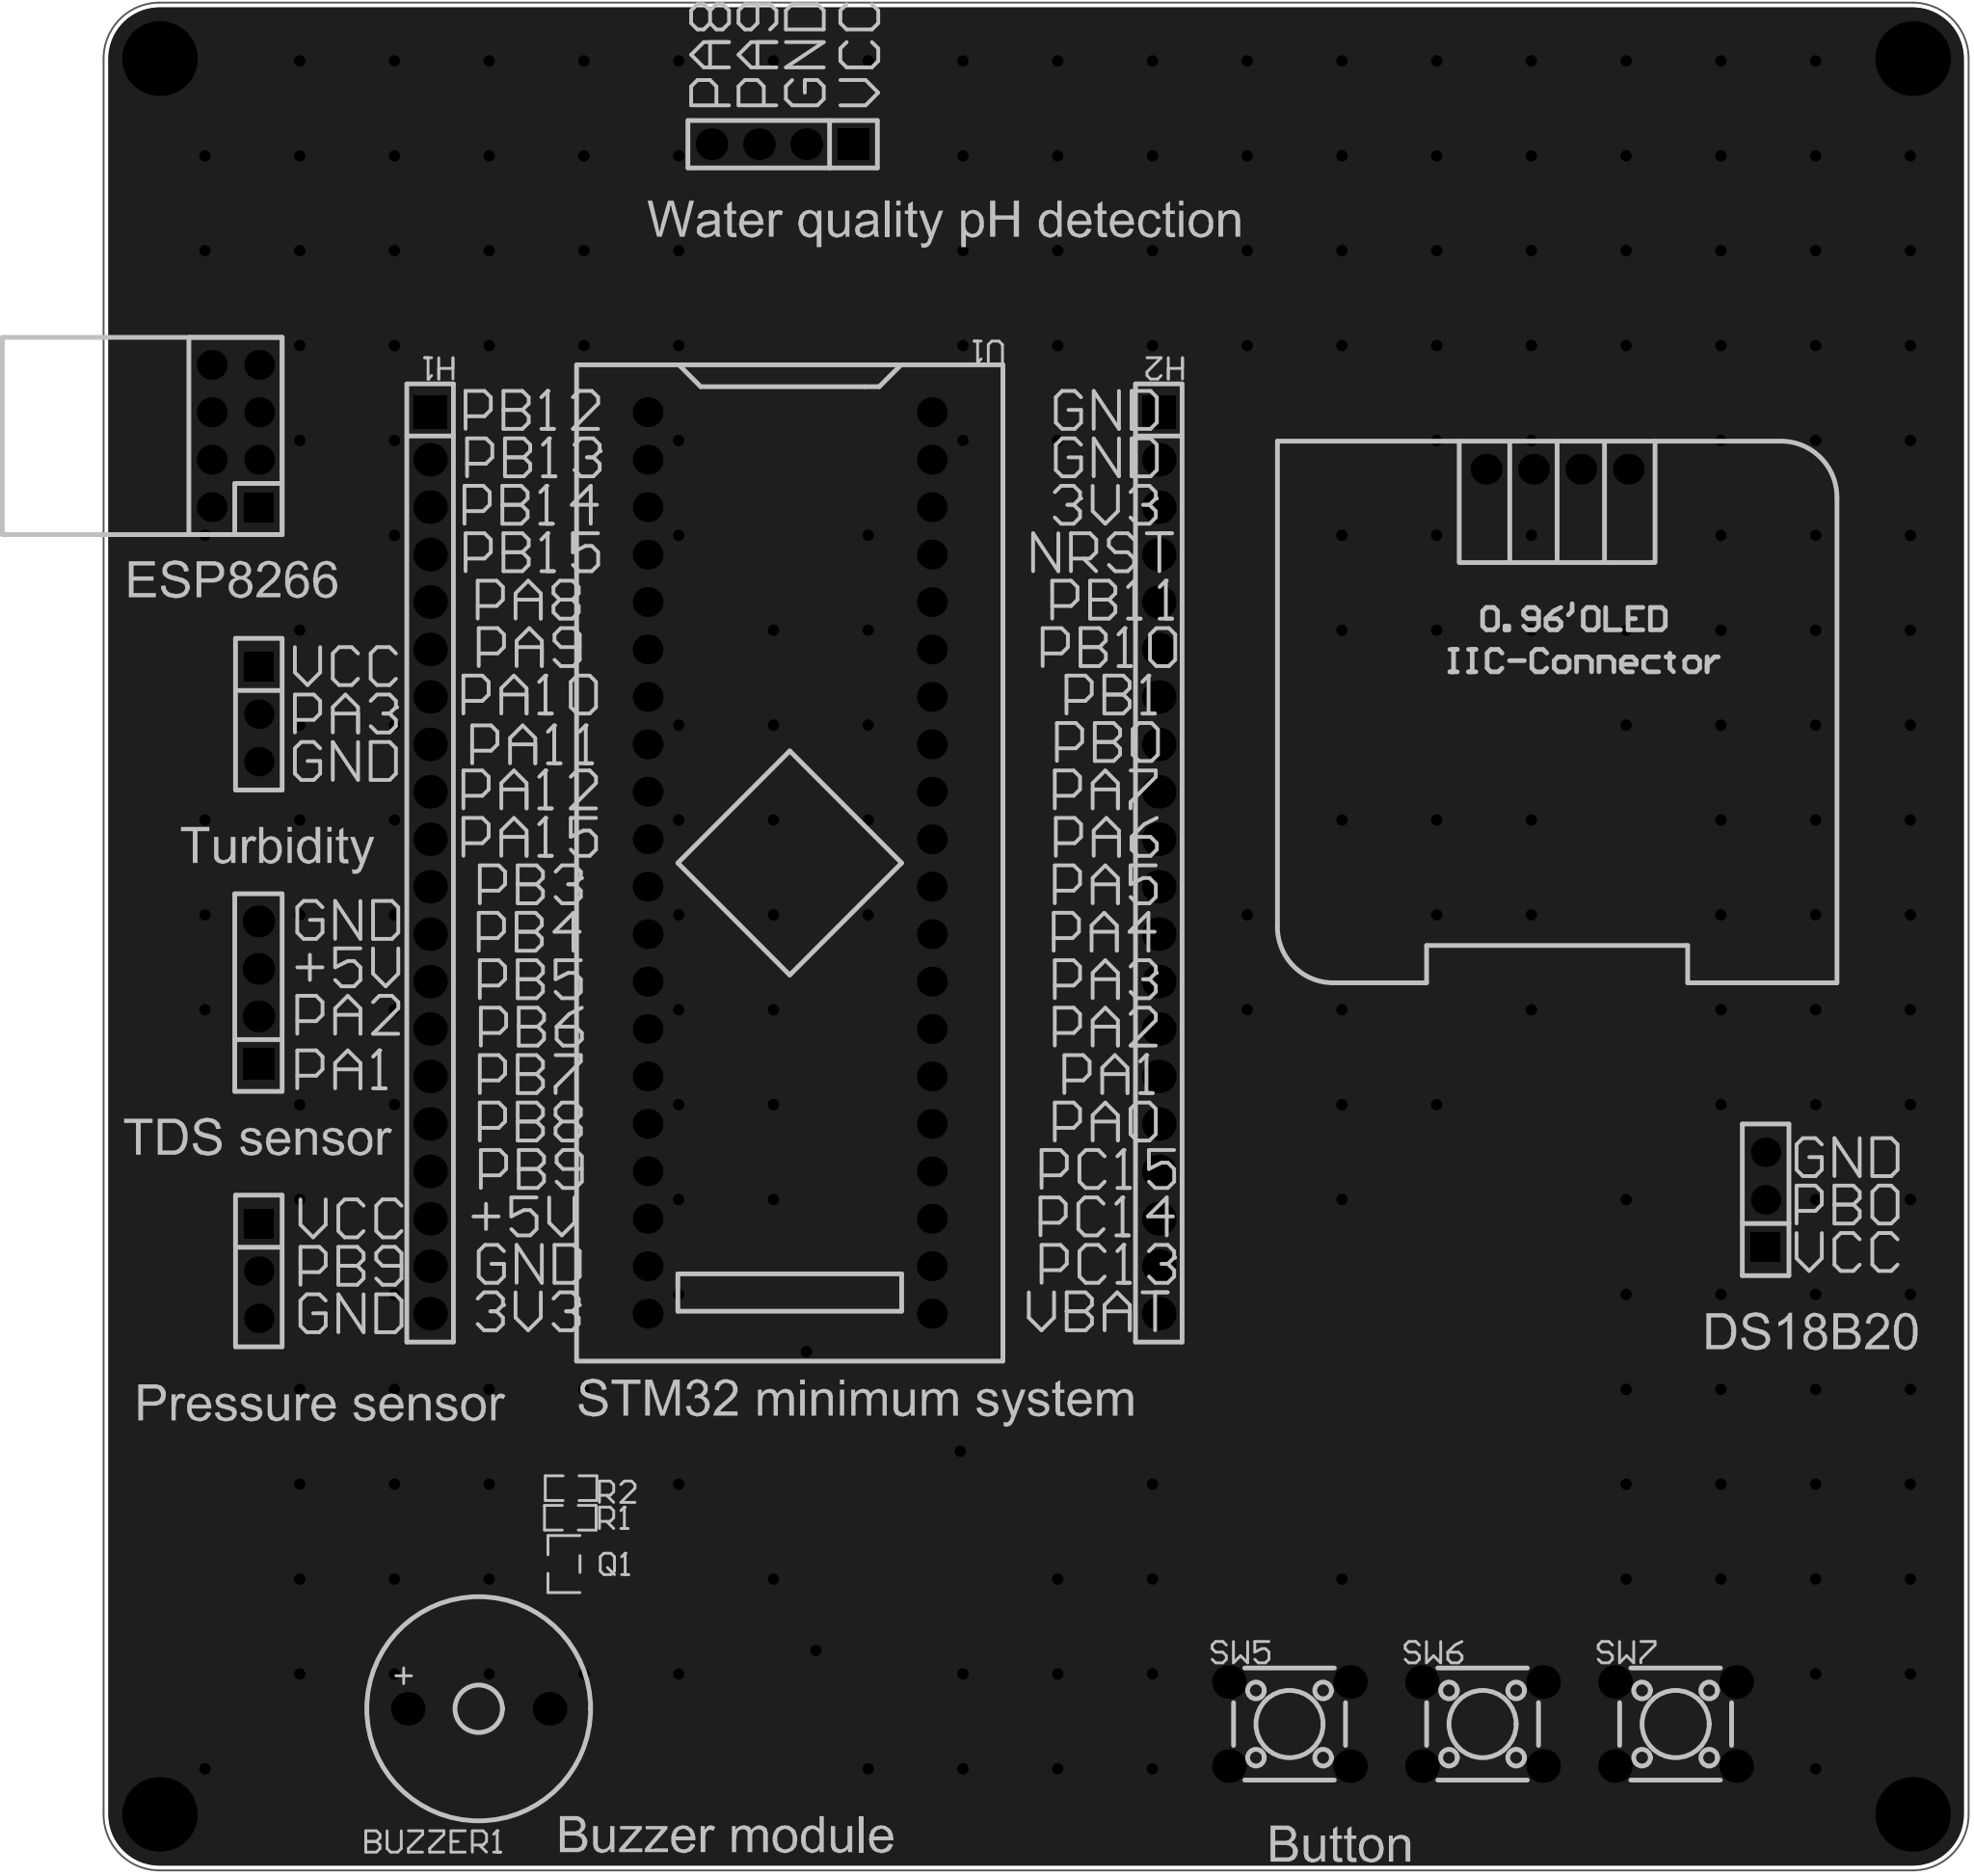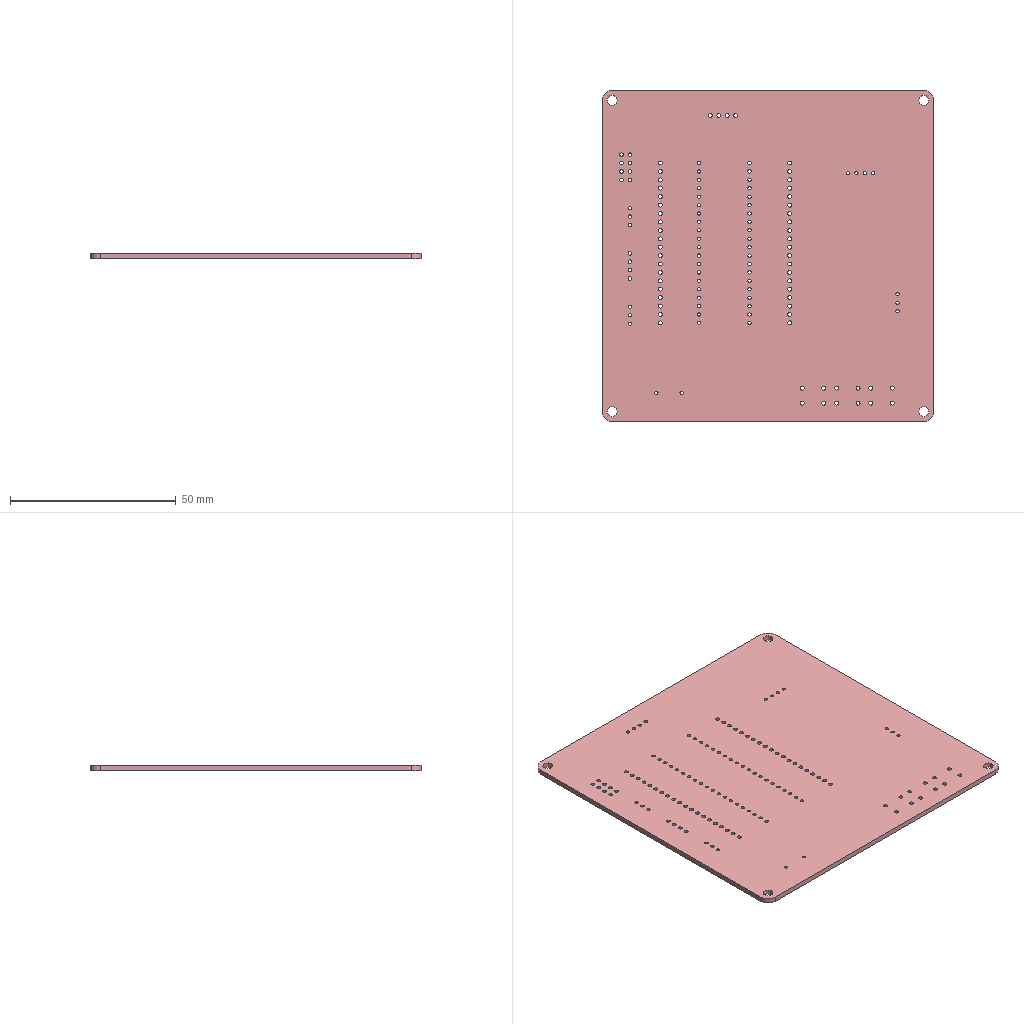Circuit board layout | Altium Designer | box 100 x 100 x 1.6 mm
Layer stack:
# Altium Designer layer stack of  (unit mm; dielectric type: 0 none, 1 core, 2 prepreg, 3 surface material)
index,name,kind,layer,copper_thickness_mm,dielectric_type,dielectric_thickness_mm,dielectric_material,dielectric_constant
0,Top Paste Mask Layer,other,,,,,,
1,Top Silkscreen Layer,other,,,,,,
2,Top Solder Mask Layer,dielectric,,,3,0.01,,3.3
3,Top Layer,copper,Top Layer,0.035,,,,
4,Dielectric1,dielectric,,,3,1.51,FR4,4.5
5,Bottom Layer,copper,Bottom Layer,0.035,,,,
6,Bottom Solder Mask Layer,dielectric,,,3,0.01,,3.3
7,Bottom Silkscreen Layer,other,,,,,,
8,Bottom Paste Mask Layer,other,,,,,,
# drill layer pairs: low layer,high layer
drill_pair,Top Layer,Bottom Layer
Part placement:
Designator,Comment,Layer,Footprint,Center-X(mm),Center-Y(mm),Rotation
U1,STM32F103C8T6-Card,TopLayer,CONN-TH_L53.3-W22.9_STM32F103C8T6-CARD,118.418,132.842,270
BUZZER1,buzzer-12X9,TopLayer,BUZ-TH_BD12.0-P7.60-D0.6-FD,101.74,87.559,0
H14,,TopLayer,HDR-TH_4P-P2.54-V-F,89.93,125.903,90
OLED1,,TopLayer,0.96OLED_4P,159.566,153.924,0
Q1,S8050 J3Y(RANGE:200-350),TopLayer,SOT-23-3_L3.0-W1.7-P0.95-LS2.9-BR,106.312,95.306,0
R1,10K,TopLayer,R0603,106.651,97.786,0
H15,,TopLayer,HDR-TH_3P-P2.54-V-F,170.742,114.808,90
H16,,TopLayer,HDR-TH_8P-P2.54-V-F-R2-C4-S2.54-1,88.7,155.702,90
H1,,TopLayer,HDR-TH_20P-P2.54-V-F,99.135,132.842,270
H2,,TopLayer,HDR-TH_20P-P2.54-V-F,138.206,132.842,270
H17,,TopLayer,HDR-TH_3P-P2.54-V-F,89.95,110.998,270
H18,,TopLayer,HDR-TH_3P-P2.54-V-F,89.95,140.807,270
R2,10K,TopLayer,R0603,106.693,99.37,180
SW5,,TopLayer,SW-TH_4P-L6.0-W6.0-P4.50-LS6.5,145.215,86.741,0
SW6,,TopLayer,SW-TH_4P-L6.0-W6.0-P4.50-LS6.5,155.565,86.741,0
SW7,,TopLayer,SW-TH_4P-L6.0-W6.0-P4.50-LS6.5,165.916,86.741,0
H20,HDR2.54-LI-2x4P,TopLayer,HDR-TH_4P-P2.54-V-M,118.037,171.323,180
Pad and via stacks:
# Altium Designer via and pad stacks of  (unit mm). Each distinct definition once, with the count of objects using it.
# via: kind,start_layer,end_layer,hole_mm,diameter_mm,mode(0 simple;1 top-mid-bottom;2 full stack),diameter_per_layer,count,example_net
# pad: kind,layer,hole_mm,hole_type(0 round;1 square;2 slot),plating,top_size,top_shape(1 round;2 rect;3 octagon;9 rounded rect),mid_size,bottom_size,mode,footprint,size_per_layer,count,example
pad,Multi-Layer,3,0,plated,4x4,1,4x4,4x4,0,,,4,1
pad,Multi-Layer,1,0,plated,1.6x1.6,1,1.6x1.6,1.6x1.6,0,CONN-TH_L53.3-W22.9_STM32F103C8T6-CARD,,40,U1.1
pad,Multi-Layer,1,0,plated,1.8x1.8,1,1.8x1.8,1.8x1.8,0,BUZ-TH_BD12.0-P7.60-D0.6-FD,,2,BUZZER1.2
pad,Multi-Layer,1.1,0,plated,1.7x1.7,2,1.7x1.7,1.7x1.7,0,HDR-TH_4P-P2.54-V-F,,1,H14.1
pad,Multi-Layer,1.1,0,plated,1.7x1.7,1,1.7x1.7,1.7x1.7,0,HDR-TH_4P-P2.54-V-F,,3,H14.2
pad,Multi-Layer,1,0,plated,1.65x1.65,1,1.65x1.65,1.65x1.65,0,0.96OLED_4P,,4,OLED1.4
pad,Multi-Layer,1.02,0,plated,1.575x1.575,1,1.575x1.575,1.575x1.575,0,HDR-TH_3P-P2.54-V-F,,6,H15.3
pad,Multi-Layer,1.02,0,plated,1.575x1.575,2,1.575x1.575,1.575x1.575,0,HDR-TH_3P-P2.54-V-F,,3,H15.1
pad,Multi-Layer,1.1,0,plated,1.6x1.6,2,1.6x1.6,1.6x1.6,0,HDR-TH_8P-P2.54-V-F-R2-C4-S2.54-1,,1,H16.1
pad,Multi-Layer,1.1,0,plated,1.6x1.6,1,1.6x1.6,1.6x1.6,0,HDR-TH_8P-P2.54-V-F-R2-C4-S2.54-1,,7,H16.2
pad,Multi-Layer,1.2,0,plated,1.8x1.8,2,1.8x1.8,1.8x1.8,0,HDR-TH_20P-P2.54-V-F,,2,H1.1
pad,Multi-Layer,1.2,0,plated,1.8x1.8,1,1.8x1.8,1.8x1.8,0,HDR-TH_20P-P2.54-V-F,,38,H1.2
pad,Multi-Layer,1.2,0,plated,1.8x1.8,1,1.8x1.8,1.8x1.8,0,SW-TH_4P-L6.0-W6.0-P4.50-LS6.5,,12,SW5.1
pad,Multi-Layer,1.1,0,plated,1.7x1.7,2,1.7x1.7,1.7x1.7,0,HDR-TH_4P-P2.54-V-M,,1,H20.1
pad,Multi-Layer,1.1,0,plated,1.7x1.7,1,1.7x1.7,1.7x1.7,0,HDR-TH_4P-P2.54-V-M,,3,H20.2
pad,Top Layer,0,0,plated,1.038x0.532,2,1.038x0.532,1.038x0.532,0,SOT-23-3_L3.0-W1.7-P0.95-LS2.9-BR,,3,Q1.1
pad,Top Layer,0,0,plated,0.8065x0.864,2,0.8065x0.864,0.8065x0.864,0,R0603,,4,R1.2
via,Top Layer,Bottom Layer,0.3048,0.61,0,,209,PA0
Copper pours:
name,layer,net,type(0 solid;1 hatched;2 none)
Bottom Layer-GND,Bottom Layer,GND,0
Top Layer-GND,Top Layer,GND,0